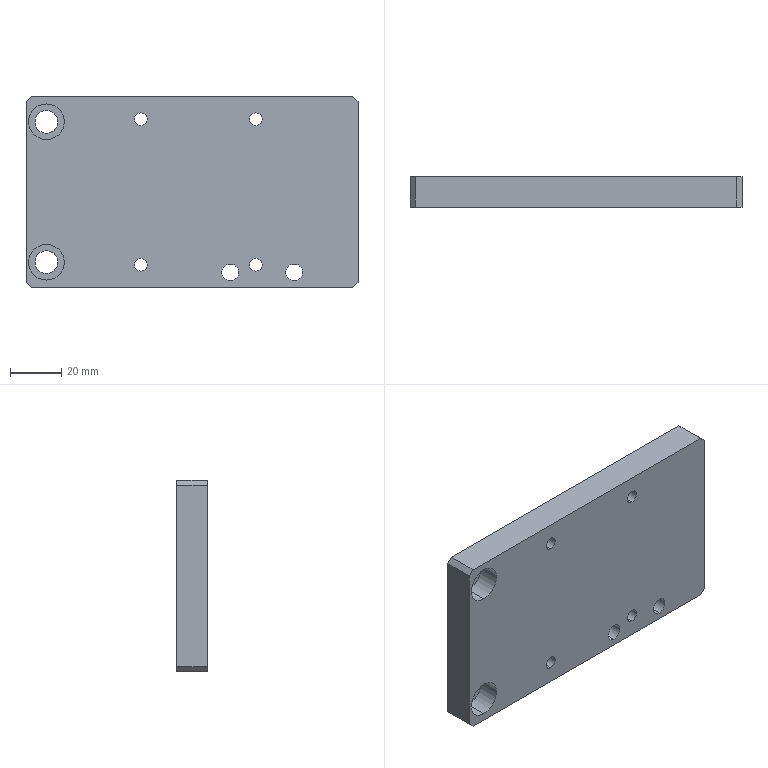Part | SolidWorks | features BaseBody 1 | 1 solid | 50 faces | box 130 x 12 x 75 mm | volume 110369 mm3 | cylinder 30 | plane 14 | cone 6 | commonest cylinder face diameters 5 x14 6.6 x4 9 x4 11 x4 14 x4
STEP:
#1=CARTESIAN_POINT('',(25.,0.,26.));
#2=VERTEX_POINT('',#1);
#3=CARTESIAN_POINT('',(25.,0.,31.));
#4=VERTEX_POINT('',#3);
#5=CARTESIAN_POINT('',(25.,0.,28.5));
#6=DIRECTION('',(0.,1.,0.));
#7=DIRECTION('',(0.,0.,1.));
#8=AXIS2_PLACEMENT_3D('',#5,#6,#7);
#9=CIRCLE('',#8,2.5);
#10=EDGE_CURVE('',#2,#4,#9,.T.);
#11=ORIENTED_EDGE('',*,*,#10,.F.);
#12=CARTESIAN_POINT('',(25.,12.,26.));
#13=VERTEX_POINT('',#12);
#14=CARTESIAN_POINT('',(25.,12.,26.));
#15=DIRECTION('',(0.,1.,0.));
#16=VECTOR('',#15,1000.);
#17=LINE('',#14,#16);
#18=EDGE_CURVE('',#2,#13,#17,.T.);
#19=ORIENTED_EDGE('',*,*,#18,.T.);
#20=CARTESIAN_POINT('',(25.,12.,31.));
#21=VERTEX_POINT('',#20);
#22=CARTESIAN_POINT('',(25.,12.,28.5));
#23=DIRECTION('',(0.,-1.,0.));
#24=DIRECTION('',(0.,0.,1.));
#25=AXIS2_PLACEMENT_3D('',#22,#23,#24);
#26=CIRCLE('',#25,2.5);
#27=EDGE_CURVE('',#21,#13,#26,.T.);
#28=ORIENTED_EDGE('',*,*,#27,.F.);
#29=CARTESIAN_POINT('',(25.,12.,31.));
#30=DIRECTION('',(0.,1.,0.));
#31=VECTOR('',#30,1000.);
#32=LINE('',#29,#31);
#33=EDGE_CURVE('',#4,#21,#32,.T.);
#34=ORIENTED_EDGE('',*,*,#33,.F.);
#35=EDGE_LOOP('',(#11,#19,#28,#34));
#36=FACE_OUTER_BOUND('',#35,.T.);
#37=CARTESIAN_POINT('',(25.,12.,28.5));
#38=DIRECTION('',(0.,1.,0.));
#39=DIRECTION('',(0.,0.,1.));
#40=AXIS2_PLACEMENT_3D('',#37,#38,#39);
#41=CYLINDRICAL_SURFACE('',#40,2.5);
#42=ADVANCED_FACE('',(#36),#41,.F.);
#43=CARTESIAN_POINT('',(-20.,0.,26.));
#44=VERTEX_POINT('',#43);
#45=CARTESIAN_POINT('',(-20.,0.,31.));
#46=VERTEX_POINT('',#45);
#47=CARTESIAN_POINT('',(-20.,0.,28.5));
#48=DIRECTION('',(0.,1.,0.));
#49=DIRECTION('',(0.,0.,1.));
#50=AXIS2_PLACEMENT_3D('',#47,#48,#49);
#51=CIRCLE('',#50,2.5);
#52=EDGE_CURVE('',#44,#46,#51,.T.);
#53=ORIENTED_EDGE('',*,*,#52,.F.);
#54=CARTESIAN_POINT('',(-20.,12.,26.));
#55=VERTEX_POINT('',#54);
#56=CARTESIAN_POINT('',(-20.,12.,26.));
#57=DIRECTION('',(0.,1.,0.));
#58=VECTOR('',#57,1000.);
#59=LINE('',#56,#58);
#60=EDGE_CURVE('',#44,#55,#59,.T.);
#61=ORIENTED_EDGE('',*,*,#60,.T.);
#62=CARTESIAN_POINT('',(-20.,12.,31.));
#63=VERTEX_POINT('',#62);
#64=CARTESIAN_POINT('',(-20.,12.,28.5));
#65=DIRECTION('',(0.,-1.,0.));
#66=DIRECTION('',(0.,0.,1.));
#67=AXIS2_PLACEMENT_3D('',#64,#65,#66);
#68=CIRCLE('',#67,2.5);
#69=EDGE_CURVE('',#63,#55,#68,.T.);
#70=ORIENTED_EDGE('',*,*,#69,.F.);
#71=CARTESIAN_POINT('',(-20.,12.,31.));
#72=DIRECTION('',(0.,1.,0.));
#73=VECTOR('',#72,1000.);
#74=LINE('',#71,#73);
#75=EDGE_CURVE('',#46,#63,#74,.T.);
#76=ORIENTED_EDGE('',*,*,#75,.F.);
#77=EDGE_LOOP('',(#53,#61,#70,#76));
#78=FACE_OUTER_BOUND('',#77,.T.);
#79=CARTESIAN_POINT('',(-20.,12.,28.5));
#80=DIRECTION('',(0.,1.,0.));
#81=DIRECTION('',(0.,0.,1.));
#82=AXIS2_PLACEMENT_3D('',#79,#80,#81);
#83=CYLINDRICAL_SURFACE('',#82,2.5);
#84=ADVANCED_FACE('',(#78),#83,.F.);
#85=CARTESIAN_POINT('',(25.,0.,-31.));
#86=VERTEX_POINT('',#85);
#87=CARTESIAN_POINT('',(25.,0.,-26.));
#88=VERTEX_POINT('',#87);
#89=CARTESIAN_POINT('',(25.,0.,-28.5));
#90=DIRECTION('',(0.,1.,0.));
#91=DIRECTION('',(0.,0.,1.));
#92=AXIS2_PLACEMENT_3D('',#89,#90,#91);
#93=CIRCLE('',#92,2.5);
#94=EDGE_CURVE('',#86,#88,#93,.T.);
#95=ORIENTED_EDGE('',*,*,#94,.F.);
#96=CARTESIAN_POINT('',(25.,12.,-31.));
#97=VERTEX_POINT('',#96);
#98=CARTESIAN_POINT('',(25.,12.,-31.));
#99=DIRECTION('',(0.,1.,0.));
#100=VECTOR('',#99,1000.);
#101=LINE('',#98,#100);
#102=EDGE_CURVE('',#86,#97,#101,.T.);
#103=ORIENTED_EDGE('',*,*,#102,.T.);
#104=CARTESIAN_POINT('',(25.,12.,-26.));
#105=VERTEX_POINT('',#104);
#106=CARTESIAN_POINT('',(25.,12.,-28.5));
#107=DIRECTION('',(0.,-1.,0.));
#108=DIRECTION('',(0.,0.,1.));
#109=AXIS2_PLACEMENT_3D('',#106,#107,#108);
#110=CIRCLE('',#109,2.5);
#111=EDGE_CURVE('',#105,#97,#110,.T.);
#112=ORIENTED_EDGE('',*,*,#111,.F.);
#113=CARTESIAN_POINT('',(25.,12.,-26.));
#114=DIRECTION('',(0.,1.,0.));
#115=VECTOR('',#114,1000.);
#116=LINE('',#113,#115);
#117=EDGE_CURVE('',#88,#105,#116,.T.);
#118=ORIENTED_EDGE('',*,*,#117,.F.);
#119=EDGE_LOOP('',(#95,#103,#112,#118));
#120=FACE_OUTER_BOUND('',#119,.T.);
#121=CARTESIAN_POINT('',(25.,12.,-28.5));
#122=DIRECTION('',(0.,1.,0.));
#123=DIRECTION('',(0.,0.,1.));
#124=AXIS2_PLACEMENT_3D('',#121,#122,#123);
#125=CYLINDRICAL_SURFACE('',#124,2.5);
#126=ADVANCED_FACE('',(#120),#125,.F.);
#127=CARTESIAN_POINT('',(-20.,0.,-31.));
#128=VERTEX_POINT('',#127);
#129=CARTESIAN_POINT('',(-20.,0.,-26.));
#130=VERTEX_POINT('',#129);
#131=CARTESIAN_POINT('',(-20.,0.,-28.5));
#132=DIRECTION('',(0.,1.,0.));
#133=DIRECTION('',(0.,0.,1.));
#134=AXIS2_PLACEMENT_3D('',#131,#132,#133);
#135=CIRCLE('',#134,2.5);
#136=EDGE_CURVE('',#128,#130,#135,.T.);
#137=ORIENTED_EDGE('',*,*,#136,.F.);
#138=CARTESIAN_POINT('',(-20.,12.,-31.));
#139=VERTEX_POINT('',#138);
#140=CARTESIAN_POINT('',(-20.,12.,-31.));
#141=DIRECTION('',(0.,1.,0.));
#142=VECTOR('',#141,1000.);
#143=LINE('',#140,#142);
#144=EDGE_CURVE('',#128,#139,#143,.T.);
#145=ORIENTED_EDGE('',*,*,#144,.T.);
#146=CARTESIAN_POINT('',(-20.,12.,-26.));
#147=VERTEX_POINT('',#146);
#148=CARTESIAN_POINT('',(-20.,12.,-28.5));
#149=DIRECTION('',(0.,-1.,0.));
#150=DIRECTION('',(0.,0.,1.));
#151=AXIS2_PLACEMENT_3D('',#148,#149,#150);
#152=CIRCLE('',#151,2.5);
#153=EDGE_CURVE('',#147,#139,#152,.T.);
#154=ORIENTED_EDGE('',*,*,#153,.F.);
#155=CARTESIAN_POINT('',(-20.,12.,-26.));
#156=DIRECTION('',(0.,1.,0.));
#157=VECTOR('',#156,1000.);
#158=LINE('',#155,#157);
#159=EDGE_CURVE('',#130,#147,#158,.T.);
#160=ORIENTED_EDGE('',*,*,#159,.F.);
#161=EDGE_LOOP('',(#137,#145,#154,#160));
#162=FACE_OUTER_BOUND('',#161,.T.);
#163=CARTESIAN_POINT('',(-20.,12.,-28.5));
#164=DIRECTION('',(0.,1.,0.));
#165=DIRECTION('',(0.,0.,1.));
#166=AXIS2_PLACEMENT_3D('',#163,#164,#165);
#167=CYLINDRICAL_SURFACE('',#166,2.5);
#168=ADVANCED_FACE('',(#162),#167,.F.);
#169=CARTESIAN_POINT('',(-57.,12.,32.));
#170=VERTEX_POINT('',#169);
#171=CARTESIAN_POINT('',(-57.,12.,23.));
#172=VERTEX_POINT('',#171);
#173=CARTESIAN_POINT('',(-57.,12.,27.5));
#174=DIRECTION('',(0.,-1.,0.));
#175=DIRECTION('',(0.,0.,-1.));
#176=AXIS2_PLACEMENT_3D('',#173,#174,#175);
#177=CIRCLE('',#176,4.5);
#178=EDGE_CURVE('',#170,#172,#177,.T.);
#179=ORIENTED_EDGE('',*,*,#178,.F.);
#180=CARTESIAN_POINT('',(-57.,8.6,32.));
#181=VERTEX_POINT('',#180);
#182=CARTESIAN_POINT('',(-57.,0.,32.));
#183=DIRECTION('',(0.,-1.,0.));
#184=VECTOR('',#183,1000.);
#185=LINE('',#182,#184);
#186=EDGE_CURVE('',#170,#181,#185,.T.);
#187=ORIENTED_EDGE('',*,*,#186,.T.);
#188=CARTESIAN_POINT('',(-57.,8.6,23.));
#189=VERTEX_POINT('',#188);
#190=CARTESIAN_POINT('',(-57.,8.6,27.5));
#191=DIRECTION('',(0.,1.,0.));
#192=DIRECTION('',(0.,0.,-1.));
#193=AXIS2_PLACEMENT_3D('',#190,#191,#192);
#194=CIRCLE('',#193,4.5);
#195=EDGE_CURVE('',#189,#181,#194,.T.);
#196=ORIENTED_EDGE('',*,*,#195,.F.);
#197=CARTESIAN_POINT('',(-57.,0.,23.));
#198=DIRECTION('',(0.,-1.,0.));
#199=VECTOR('',#198,1000.);
#200=LINE('',#197,#199);
#201=EDGE_CURVE('',#172,#189,#200,.T.);
#202=ORIENTED_EDGE('',*,*,#201,.F.);
#203=EDGE_LOOP('',(#179,#187,#196,#202));
#204=FACE_OUTER_BOUND('',#203,.T.);
#205=CARTESIAN_POINT('',(-57.,0.,27.5));
#206=DIRECTION('',(0.,-1.,0.));
#207=DIRECTION('',(0.,0.,-1.));
#208=AXIS2_PLACEMENT_3D('',#205,#206,#207);
#209=CYLINDRICAL_SURFACE('',#208,4.5);
#210=ADVANCED_FACE('',(#204),#209,.F.);
#211=CARTESIAN_POINT('',(-57.,12.,-23.));
#212=VERTEX_POINT('',#211);
#213=CARTESIAN_POINT('',(-57.,12.,-32.));
#214=VERTEX_POINT('',#213);
#215=CARTESIAN_POINT('',(-57.,12.,-27.5));
#216=DIRECTION('',(0.,-1.,0.));
#217=DIRECTION('',(0.,0.,-1.));
#218=AXIS2_PLACEMENT_3D('',#215,#216,#217);
#219=CIRCLE('',#218,4.5);
#220=EDGE_CURVE('',#212,#214,#219,.T.);
#221=ORIENTED_EDGE('',*,*,#220,.F.);
#222=CARTESIAN_POINT('',(-57.,8.6,-23.));
#223=VERTEX_POINT('',#222);
#224=CARTESIAN_POINT('',(-57.,0.,-23.));
#225=DIRECTION('',(0.,-1.,0.));
#226=VECTOR('',#225,1000.);
#227=LINE('',#224,#226);
#228=EDGE_CURVE('',#212,#223,#227,.T.);
#229=ORIENTED_EDGE('',*,*,#228,.T.);
#230=CARTESIAN_POINT('',(-57.,8.6,-32.));
#231=VERTEX_POINT('',#230);
#232=CARTESIAN_POINT('',(-57.,8.6,-27.5));
#233=DIRECTION('',(0.,1.,0.));
#234=DIRECTION('',(0.,0.,-1.));
#235=AXIS2_PLACEMENT_3D('',#232,#233,#234);
#236=CIRCLE('',#235,4.5);
#237=EDGE_CURVE('',#231,#223,#236,.T.);
#238=ORIENTED_EDGE('',*,*,#237,.F.);
#239=CARTESIAN_POINT('',(-57.,0.,-32.));
#240=DIRECTION('',(0.,-1.,0.));
#241=VECTOR('',#240,1000.);
#242=LINE('',#239,#241);
#243=EDGE_CURVE('',#214,#231,#242,.T.);
#244=ORIENTED_EDGE('',*,*,#243,.F.);
#245=EDGE_LOOP('',(#221,#229,#238,#244));
#246=FACE_OUTER_BOUND('',#245,.T.);
#247=CARTESIAN_POINT('',(-57.,0.,-27.5));
#248=DIRECTION('',(0.,-1.,0.));
#249=DIRECTION('',(0.,0.,-1.));
#250=AXIS2_PLACEMENT_3D('',#247,#248,#249);
#251=CYLINDRICAL_SURFACE('',#250,4.5);
#252=ADVANCED_FACE('',(#246),#251,.F.);
#253=CARTESIAN_POINT('',(40.,5.6,-37.));
#254=VERTEX_POINT('',#253);
#255=CARTESIAN_POINT('',(40.,5.6,-26.));
#256=VERTEX_POINT('',#255);
#257=CARTESIAN_POINT('',(40.,5.6,-31.5));
#258=DIRECTION('',(0.,1.,0.));
#259=DIRECTION('',(0.,0.,1.));
#260=AXIS2_PLACEMENT_3D('',#257,#258,#259);
#261=CIRCLE('',#260,5.5);
#262=EDGE_CURVE('',#254,#256,#261,.T.);
#263=ORIENTED_EDGE('',*,*,#262,.F.);
#264=CARTESIAN_POINT('',(40.,12.,-37.));
#265=VERTEX_POINT('',#264);
#266=CARTESIAN_POINT('',(40.,12.,-37.));
#267=DIRECTION('',(0.,1.,0.));
#268=VECTOR('',#267,1000.);
#269=LINE('',#266,#268);
#270=EDGE_CURVE('',#254,#265,#269,.T.);
#271=ORIENTED_EDGE('',*,*,#270,.T.);
#272=CARTESIAN_POINT('',(40.,12.,-26.));
#273=VERTEX_POINT('',#272);
#274=CARTESIAN_POINT('',(40.,12.,-31.5));
#275=DIRECTION('',(0.,-1.,0.));
#276=DIRECTION('',(0.,0.,1.));
#277=AXIS2_PLACEMENT_3D('',#274,#275,#276);
#278=CIRCLE('',#277,5.5);
#279=EDGE_CURVE('',#273,#265,#278,.T.);
#280=ORIENTED_EDGE('',*,*,#279,.F.);
#281=CARTESIAN_POINT('',(40.,12.,-26.));
#282=DIRECTION('',(0.,1.,0.));
#283=VECTOR('',#282,1000.);
#284=LINE('',#281,#283);
#285=EDGE_CURVE('',#256,#273,#284,.T.);
#286=ORIENTED_EDGE('',*,*,#285,.F.);
#287=EDGE_LOOP('',(#263,#271,#280,#286));
#288=FACE_OUTER_BOUND('',#287,.T.);
#289=CARTESIAN_POINT('',(40.,12.,-31.5));
#290=DIRECTION('',(0.,1.,0.));
#291=DIRECTION('',(0.,0.,1.));
#292=AXIS2_PLACEMENT_3D('',#289,#290,#291);
#293=CYLINDRICAL_SURFACE('',#292,5.5);
#294=ADVANCED_FACE('',(#288),#293,.F.);
#295=CARTESIAN_POINT('',(15.,5.6,-37.));
#296=VERTEX_POINT('',#295);
#297=CARTESIAN_POINT('',(15.,5.6,-26.));
#298=VERTEX_POINT('',#297);
#299=CARTESIAN_POINT('',(15.,5.6,-31.5));
#300=DIRECTION('',(0.,1.,0.));
#301=DIRECTION('',(0.,0.,1.));
#302=AXIS2_PLACEMENT_3D('',#299,#300,#301);
#303=CIRCLE('',#302,5.5);
#304=EDGE_CURVE('',#296,#298,#303,.T.);
#305=ORIENTED_EDGE('',*,*,#304,.F.);
#306=CARTESIAN_POINT('',(15.,12.,-37.));
#307=VERTEX_POINT('',#306);
#308=CARTESIAN_POINT('',(15.,12.,-37.));
#309=DIRECTION('',(0.,1.,0.));
#310=VECTOR('',#309,1000.);
#311=LINE('',#308,#310);
#312=EDGE_CURVE('',#296,#307,#311,.T.);
#313=ORIENTED_EDGE('',*,*,#312,.T.);
#314=CARTESIAN_POINT('',(15.,12.,-26.));
#315=VERTEX_POINT('',#314);
#316=CARTESIAN_POINT('',(15.,12.,-31.5));
#317=DIRECTION('',(0.,-1.,0.));
#318=DIRECTION('',(0.,0.,1.));
#319=AXIS2_PLACEMENT_3D('',#316,#317,#318);
#320=CIRCLE('',#319,5.5);
#321=EDGE_CURVE('',#315,#307,#320,.T.);
#322=ORIENTED_EDGE('',*,*,#321,.F.);
#323=CARTESIAN_POINT('',(15.,12.,-26.));
#324=DIRECTION('',(0.,1.,0.));
#325=VECTOR('',#324,1000.);
#326=LINE('',#323,#325);
#327=EDGE_CURVE('',#298,#315,#326,.T.);
#328=ORIENTED_EDGE('',*,*,#327,.F.);
#329=EDGE_LOOP('',(#305,#313,#322,#328));
#330=FACE_OUTER_BOUND('',#329,.T.);
#331=CARTESIAN_POINT('',(15.,12.,-31.5));
#332=DIRECTION('',(0.,1.,0.));
#333=DIRECTION('',(0.,0.,1.));
#334=AXIS2_PLACEMENT_3D('',#331,#332,#333);
#335=CYLINDRICAL_SURFACE('',#334,5.5);
#336=ADVANCED_FACE('',(#330),#335,.F.);
#337=CARTESIAN_POINT('',(50.,6.,-22.5));
#338=VERTEX_POINT('',#337);
#339=CARTESIAN_POINT('',(50.,6.,-27.5));
#340=VERTEX_POINT('',#339);
#341=CARTESIAN_POINT('',(50.,6.,-25.));
#342=DIRECTION('',(1.,0.,0.));
#343=DIRECTION('',(0.,0.,-1.));
#344=AXIS2_PLACEMENT_3D('',#341,#342,#343);
#345=CIRCLE('',#344,2.5);
#346=EDGE_CURVE('',#338,#340,#345,.T.);
#347=ORIENTED_EDGE('',*,*,#346,.F.);
#348=CARTESIAN_POINT('',(65.,6.,-22.5));
#349=VERTEX_POINT('',#348);
#350=CARTESIAN_POINT('',(65.,6.,-22.5));
#351=DIRECTION('',(1.,0.,0.));
#352=VECTOR('',#351,1000.);
#353=LINE('',#350,#352);
#354=EDGE_CURVE('',#338,#349,#353,.T.);
#355=ORIENTED_EDGE('',*,*,#354,.T.);
#356=CARTESIAN_POINT('',(65.,6.,-27.5));
#357=VERTEX_POINT('',#356);
#358=CARTESIAN_POINT('',(65.,6.,-25.));
#359=DIRECTION('',(1.,0.,0.));
#360=DIRECTION('',(0.,0.,-1.));
#361=AXIS2_PLACEMENT_3D('',#358,#359,#360);
#362=CIRCLE('',#361,2.5);
#363=EDGE_CURVE('',#349,#357,#362,.T.);
#364=ORIENTED_EDGE('',*,*,#363,.T.);
#365=CARTESIAN_POINT('',(65.,6.,-27.5));
#366=DIRECTION('',(1.,0.,0.));
#367=VECTOR('',#366,1000.);
#368=LINE('',#365,#367);
#369=EDGE_CURVE('',#340,#357,#368,.T.);
#370=ORIENTED_EDGE('',*,*,#369,.F.);
#371=EDGE_LOOP('',(#347,#355,#364,#370));
#372=FACE_OUTER_BOUND('',#371,.T.);
#373=CARTESIAN_POINT('',(65.,6.,-25.));
#374=DIRECTION('',(1.,0.,0.));
#375=DIRECTION('',(0.,0.,-1.));
#376=AXIS2_PLACEMENT_3D('',#373,#374,#375);
#377=CYLINDRICAL_SURFACE('',#376,2.5);
#378=ADVANCED_FACE('',(#372),#377,.F.);
#379=CARTESIAN_POINT('',(50.,6.,2.5));
#380=VERTEX_POINT('',#379);
#381=CARTESIAN_POINT('',(50.,6.,-2.5));
#382=VERTEX_POINT('',#381);
#383=CARTESIAN_POINT('',(50.,6.,0.));
#384=DIRECTION('',(1.,0.,0.));
#385=DIRECTION('',(0.,0.,-1.));
#386=AXIS2_PLACEMENT_3D('',#383,#384,#385);
#387=CIRCLE('',#386,2.5);
#388=EDGE_CURVE('',#380,#382,#387,.T.);
#389=ORIENTED_EDGE('',*,*,#388,.F.);
#390=CARTESIAN_POINT('',(65.,6.,2.5));
#391=VERTEX_POINT('',#390);
#392=CARTESIAN_POINT('',(65.,6.,2.5));
#393=DIRECTION('',(1.,0.,0.));
#394=VECTOR('',#393,1000.);
#395=LINE('',#392,#394);
#396=EDGE_CURVE('',#380,#391,#395,.T.);
#397=ORIENTED_EDGE('',*,*,#396,.T.);
#398=CARTESIAN_POINT('',(65.,6.,-2.5));
#399=VERTEX_POINT('',#398);
#400=CARTESIAN_POINT('',(65.,6.,0.));
#401=DIRECTION('',(1.,0.,0.));
#402=DIRECTION('',(0.,0.,-1.));
#403=AXIS2_PLACEMENT_3D('',#400,#401,#402);
#404=CIRCLE('',#403,2.5);
#405=EDGE_CURVE('',#391,#399,#404,.T.);
#406=ORIENTED_EDGE('',*,*,#405,.T.);
#407=CARTESIAN_POINT('',(65.,6.,-2.5));
#408=DIRECTION('',(1.,0.,0.));
#409=VECTOR('',#408,1000.);
#410=LINE('',#407,#409);
#411=EDGE_CURVE('',#382,#399,#410,.T.);
#412=ORIENTED_EDGE('',*,*,#411,.F.);
#413=EDGE_LOOP('',(#389,#397,#406,#412));
#414=FACE_OUTER_BOUND('',#413,.T.);
#415=CARTESIAN_POINT('',(65.,6.,0.));
#416=DIRECTION('',(1.,0.,0.));
#417=DIRECTION('',(0.,0.,-1.));
#418=AXIS2_PLACEMENT_3D('',#415,#416,#417);
#419=CYLINDRICAL_SURFACE('',#418,2.5);
#420=ADVANCED_FACE('',(#414),#419,.F.);
#421=CARTESIAN_POINT('',(50.,6.,27.5));
#422=VERTEX_POINT('',#421);
#423=CARTESIAN_POINT('',(50.,6.,22.5));
#424=VERTEX_POINT('',#423);
#425=CARTESIAN_POINT('',(50.,6.,25.));
#426=DIRECTION('',(1.,0.,0.));
#427=DIRECTION('',(0.,0.,-1.));
#428=AXIS2_PLACEMENT_3D('',#425,#426,#427);
#429=CIRCLE('',#428,2.5);
#430=EDGE_CURVE('',#422,#424,#429,.T.);
#431=ORIENTED_EDGE('',*,*,#430,.F.);
#432=CARTESIAN_POINT('',(65.,6.,27.5));
#433=VERTEX_POINT('',#432);
#434=CARTESIAN_POINT('',(65.,6.,27.5));
#435=DIRECTION('',(1.,0.,0.));
#436=VECTOR('',#435,1000.);
#437=LINE('',#434,#436);
#438=EDGE_CURVE('',#422,#433,#437,.T.);
#439=ORIENTED_EDGE('',*,*,#438,.T.);
#440=CARTESIAN_POINT('',(65.,6.,22.5));
#441=VERTEX_POINT('',#440);
#442=CARTESIAN_POINT('',(65.,6.,25.));
#443=DIRECTION('',(1.,0.,0.));
#444=DIRECTION('',(0.,0.,-1.));
#445=AXIS2_PLACEMENT_3D('',#442,#443,#444);
#446=CIRCLE('',#445,2.5);
#447=EDGE_CURVE('',#433,#441,#446,.T.);
#448=ORIENTED_EDGE('',*,*,#447,.T.);
#449=CARTESIAN_POINT('',(65.,6.,22.5));
#450=DIRECTION('',(1.,0.,0.));
#451=VECTOR('',#450,1000.);
#452=LINE('',#449,#451);
#453=EDGE_CURVE('',#424,#441,#452,.T.);
#454=ORIENTED_EDGE('',*,*,#453,.F.);
#455=EDGE_LOOP('',(#431,#439,#448,#454));
#456=FACE_OUTER_BOUND('',#455,.T.);
#457=CARTESIAN_POINT('',(65.,6.,25.));
#458=DIRECTION('',(1.,0.,0.));
#459=DIRECTION('',(0.,0.,-1.));
#460=AXIS2_PLACEMENT_3D('',#457,#458,#459);
#461=CYLINDRICAL_SURFACE('',#460,2.5);
#462=ADVANCED_FACE('',(#456),#461,.F.);
#463=CARTESIAN_POINT('',(-57.,8.6,20.5));
#464=VERTEX_POINT('',#463);
#465=CARTESIAN_POINT('',(-57.,8.6,34.5));
#466=VERTEX_POINT('',#465);
#467=CARTESIAN_POINT('',(-57.,8.6,27.5));
#468=DIRECTION('',(0.,1.,0.));
#469=DIRECTION('',(0.,0.,-1.));
#470=AXIS2_PLACEMENT_3D('',#467,#468,#469);
#471=CIRCLE('',#470,7.);
#472=EDGE_CURVE('',#464,#466,#471,.T.);
#473=ORIENTED_EDGE('',*,*,#472,.T.);
#474=CARTESIAN_POINT('',(-57.,0.,34.5));
#475=VERTEX_POINT('',#474);
#476=CARTESIAN_POINT('',(-57.,0.,34.5));
#477=DIRECTION('',(0.,-1.,0.));
#478=VECTOR('',#477,1000.);
#479=LINE('',#476,#478);
#480=EDGE_CURVE('',#466,#475,#479,.T.);
#481=ORIENTED_EDGE('',*,*,#480,.T.);
#482=CARTESIAN_POINT('',(-57.,0.,20.5));
#483=VERTEX_POINT('',#482);
#484=CARTESIAN_POINT('',(-57.,0.,27.5));
#485=DIRECTION('',(0.,-1.,0.));
#486=DIRECTION('',(0.,0.,-1.));
#487=AXIS2_PLACEMENT_3D('',#484,#485,#486);
#488=CIRCLE('',#487,7.);
#489=EDGE_CURVE('',#475,#483,#488,.T.);
#490=ORIENTED_EDGE('',*,*,#489,.T.);
#491=CARTESIAN_POINT('',(-57.,0.,20.5));
#492=DIRECTION('',(0.,-1.,0.));
#493=VECTOR('',#492,1000.);
#494=LINE('',#491,#493);
#495=EDGE_CURVE('',#464,#483,#494,.T.);
#496=ORIENTED_EDGE('',*,*,#495,.F.);
#497=EDGE_LOOP('',(#473,#481,#490,#496));
#498=FACE_OUTER_BOUND('',#497,.T.);
#499=CARTESIAN_POINT('',(-57.,0.,27.5));
#500=DIRECTION('',(0.,-1.,0.));
#501=DIRECTION('',(0.,0.,-1.));
#502=AXIS2_PLACEMENT_3D('',#499,#500,#501);
#503=CYLINDRICAL_SURFACE('',#502,7.);
#504=ADVANCED_FACE('',(#498),#503,.F.);
#505=CARTESIAN_POINT('',(-57.,8.6,-34.5));
#506=VERTEX_POINT('',#505);
#507=CARTESIAN_POINT('',(-57.,8.6,-20.5));
#508=VERTEX_POINT('',#507);
#509=CARTESIAN_POINT('',(-57.,8.6,-27.5));
#510=DIRECTION('',(0.,1.,0.));
#511=DIRECTION('',(0.,0.,-1.));
#512=AXIS2_PLACEMENT_3D('',#509,#510,#511);
#513=CIRCLE('',#512,7.);
#514=EDGE_CURVE('',#506,#508,#513,.T.);
#515=ORIENTED_EDGE('',*,*,#514,.T.);
#516=CARTESIAN_POINT('',(-57.,0.,-20.5));
#517=VERTEX_POINT('',#516);
#518=CARTESIAN_POINT('',(-57.,0.,-20.5));
#519=DIRECTION('',(0.,-1.,0.));
#520=VECTOR('',#519,1000.);
#521=LINE('',#518,#520);
#522=EDGE_CURVE('',#508,#517,#521,.T.);
#523=ORIENTED_EDGE('',*,*,#522,.T.);
#524=CARTESIAN_POINT('',(-57.,0.,-34.5));
#525=VERTEX_POINT('',#524);
#526=CARTESIAN_POINT('',(-57.,0.,-27.5));
#527=DIRECTION('',(0.,-1.,0.));
#528=DIRECTION('',(0.,0.,-1.));
#529=AXIS2_PLACEMENT_3D('',#526,#527,#528);
#530=CIRCLE('',#529,7.);
#531=EDGE_CURVE('',#517,#525,#530,.T.);
#532=ORIENTED_EDGE('',*,*,#531,.T.);
#533=CARTESIAN_POINT('',(-57.,0.,-34.5));
#534=DIRECTION('',(0.,-1.,0.));
#535=VECTOR('',#534,1000.);
#536=LINE('',#533,#535);
#537=EDGE_CURVE('',#506,#525,#536,.T.);
#538=ORIENTED_EDGE('',*,*,#537,.F.);
#539=EDGE_LOOP('',(#515,#523,#532,#538));
#540=FACE_OUTER_BOUND('',#539,.T.);
#541=CARTESIAN_POINT('',(-57.,0.,-27.5));
#542=DIRECTION('',(0.,-1.,0.));
#543=DIRECTION('',(0.,0.,-1.));
#544=AXIS2_PLACEMENT_3D('',#541,#542,#543);
#545=CYLINDRICAL_SURFACE('',#544,7.);
#546=ADVANCED_FACE('',(#540),#545,.F.);
#547=CARTESIAN_POINT('',(40.,0.,-28.2));
#548=VERTEX_POINT('',#547);
#549=CARTESIAN_POINT('',(40.,0.,-34.8));
#550=VERTEX_POINT('',#549);
#551=CARTESIAN_POINT('',(40.,0.,-31.5));
#552=DIRECTION('',(0.,-1.,0.));
#553=DIRECTION('',(0.,0.,1.));
#554=AXIS2_PLACEMENT_3D('',#551,#552,#553);
#555=CIRCLE('',#554,3.3);
#556=EDGE_CURVE('',#548,#550,#555,.T.);
#557=ORIENTED_EDGE('',*,*,#556,.T.);
#558=CARTESIAN_POINT('',(40.,5.6,-34.8));
#559=VERTEX_POINT('',#558);
#560=CARTESIAN_POINT('',(40.,12.,-34.8));
#561=DIRECTION('',(0.,1.,0.));
#562=VECTOR('',#561,1000.);
#563=LINE('',#560,#562);
#564=EDGE_CURVE('',#550,#559,#563,.T.);
#565=ORIENTED_EDGE('',*,*,#564,.T.);
#566=CARTESIAN_POINT('',(40.,5.6,-28.2));
#567=VERTEX_POINT('',#566);
#568=CARTESIAN_POINT('',(40.,5.6,-31.5));
#569=DIRECTION('',(0.,1.,0.));
#570=DIRECTION('',(0.,0.,1.));
#571=AXIS2_PLACEMENT_3D('',#568,#569,#570);
#572=CIRCLE('',#571,3.3);
#573=EDGE_CURVE('',#559,#567,#572,.T.);
#574=ORIENTED_EDGE('',*,*,#573,.T.);
#575=CARTESIAN_POINT('',(40.,12.,-28.2));
#576=DIRECTION('',(0.,1.,0.));
#577=VECTOR('',#576,1000.);
#578=LINE('',#575,#577);
#579=EDGE_CURVE('',#548,#567,#578,.T.);
#580=ORIENTED_EDGE('',*,*,#579,.F.);
#581=EDGE_LOOP('',(#557,#565,#574,#580));
#582=FACE_OUTER_BOUND('',#581,.T.);
#583=CARTESIAN_POINT('',(40.,12.,-31.5));
#584=DIRECTION('',(0.,1.,0.));
#585=DIRECTION('',(0.,0.,1.));
#586=AXIS2_PLACEMENT_3D('',#583,#584,#585);
#587=CYLINDRICAL_SURFACE('',#586,3.3);
#588=ADVANCED_FACE('',(#582),#587,.F.);
#589=CARTESIAN_POINT('',(15.,0.,-28.2));
#590=VERTEX_POINT('',#589);
#591=CARTESIAN_POINT('',(15.,0.,-34.8));
#592=VERTEX_POINT('',#591);
#593=CARTESIAN_POINT('',(15.,0.,-31.5));
#594=DIRECTION('',(0.,-1.,0.));
#595=DIRECTION('',(0.,0.,1.));
#596=AXIS2_PLACEMENT_3D('',#593,#594,#595);
#597=CIRCLE('',#596,3.3);
#598=EDGE_CURVE('',#590,#592,#597,.T.);
#599=ORIENTED_EDGE('',*,*,#598,.T.);
#600=CARTESIAN_POINT('',(15.,5.6,-34.8));
#601=VERTEX_POINT('',#600);
#602=CARTESIAN_POINT('',(15.,12.,-34.8));
#603=DIRECTION('',(0.,1.,0.));
#604=VECTOR('',#603,1000.);
#605=LINE('',#602,#604);
#606=EDGE_CURVE('',#592,#601,#605,.T.);
#607=ORIENTED_EDGE('',*,*,#606,.T.);
#608=CARTESIAN_POINT('',(15.,5.6,-28.2));
#609=VERTEX_POINT('',#608);
#610=CARTESIAN_POINT('',(15.,5.6,-31.5));
#611=DIRECTION('',(0.,1.,0.));
#612=DIRECTION('',(0.,0.,1.));
#613=AXIS2_PLACEMENT_3D('',#610,#611,#612);
#614=CIRCLE('',#613,3.3);
#615=EDGE_CURVE('',#601,#609,#614,.T.);
#616=ORIENTED_EDGE('',*,*,#615,.T.);
#617=CARTESIAN_POINT('',(15.,12.,-28.2));
#618=DIRECTION('',(0.,1.,0.));
#619=VECTOR('',#618,1000.);
#620=LINE('',#617,#619);
#621=EDGE_CURVE('',#590,#609,#620,.T.);
#622=ORIENTED_EDGE('',*,*,#621,.F.);
#623=EDGE_LOOP('',(#599,#607,#616,#622));
#624=FACE_OUTER_BOUND('',#623,.T.);
#625=CARTESIAN_POINT('',(15.,12.,-31.5));
#626=DIRECTION('',(0.,1.,0.));
#627=DIRECTION('',(0.,0.,1.));
#628=AXIS2_PLACEMENT_3D('',#625,#626,#627);
#629=CYLINDRICAL_SURFACE('',#628,3.3);
#630=ADVANCED_FACE('',(#624),#629,.F.);
#631=CARTESIAN_POINT('',(48.498,6.,-25.));
#632=VERTEX_POINT('',#631);
#633=CARTESIAN_POINT('',(50.,6.,-27.5));
#634=DIRECTION('',(0.515,0.,-0.8572));
#635=VECTOR('',#634,1000.);
#636=LINE('',#633,#635);
#637=EDGE_CURVE('',#632,#340,#636,.T.);
#638=ORIENTED_EDGE('',*,*,#637,.F.);
#639=CARTESIAN_POINT('',(50.,6.,-22.5));
#640=DIRECTION('',(0.515,0.,0.8572));
#641=VECTOR('',#640,1000.);
#642=LINE('',#639,#641);
#643=EDGE_CURVE('',#632,#338,#642,.T.);
#644=ORIENTED_EDGE('',*,*,#643,.T.);
#645=ORIENTED_EDGE('',*,*,#346,.T.);
#646=EDGE_LOOP('',(#638,#644,#645));
#647=FACE_OUTER_BOUND('',#646,.T.);
#648=CARTESIAN_POINT('',(50.,6.,-25.));
#649=DIRECTION('',(1.,0.,0.));
#650=DIRECTION('',(0.,0.,-1.));
#651=AXIS2_PLACEMENT_3D('',#648,#649,#650);
#652=CONICAL_SURFACE('',#651,2.5,1.03);
#653=ADVANCED_FACE('',(#647),#652,.F.);
#654=CARTESIAN_POINT('',(48.498,6.,0.));
#655=VERTEX_POINT('',#654);
#656=CARTESIAN_POINT('',(50.,6.,-2.5));
#657=DIRECTION('',(0.515,0.,-0.8572));
#658=VECTOR('',#657,1000.);
#659=LINE('',#656,#658);
#660=EDGE_CURVE('',#655,#382,#659,.T.);
#661=ORIENTED_EDGE('',*,*,#660,.F.);
#662=CARTESIAN_POINT('',(50.,6.,2.5));
#663=DIRECTION('',(0.515,0.,0.8572));
#664=VECTOR('',#663,1000.);
#665=LINE('',#662,#664);
#666=EDGE_CURVE('',#655,#380,#665,.T.);
#667=ORIENTED_EDGE('',*,*,#666,.T.);
#668=ORIENTED_EDGE('',*,*,#388,.T.);
#669=EDGE_LOOP('',(#661,#667,#668));
#670=FACE_OUTER_BOUND('',#669,.T.);
#671=CARTESIAN_POINT('',(50.,6.,0.));
#672=DIRECTION('',(1.,0.,0.));
#673=DIRECTION('',(0.,0.,-1.));
#674=AXIS2_PLACEMENT_3D('',#671,#672,#673);
#675=CONICAL_SURFACE('',#674,2.5,1.03);
#676=ADVANCED_FACE('',(#670),#675,.F.);
#677=CARTESIAN_POINT('',(48.498,6.,25.));
#678=VERTEX_POINT('',#677);
#679=CARTESIAN_POINT('',(50.,6.,22.5));
#680=DIRECTION('',(0.515,0.,-0.8572));
#681=VECTOR('',#680,1000.);
#682=LINE('',#679,#681);
#683=EDGE_CURVE('',#678,#424,#682,.T.);
#684=ORIENTED_EDGE('',*,*,#683,.F.);
#685=CARTESIAN_POINT('',(50.,6.,27.5));
#686=DIRECTION('',(0.515,0.,0.8572));
#687=VECTOR('',#686,1000.);
#688=LINE('',#685,#687);
#689=EDGE_CURVE('',#678,#422,#688,.T.);
#690=ORIENTED_EDGE('',*,*,#689,.T.);
#691=ORIENTED_EDGE('',*,*,#430,.T.);
#692=EDGE_LOOP('',(#684,#690,#691));
#693=FACE_OUTER_BOUND('',#692,.T.);
#694=CARTESIAN_POINT('',(50.,6.,25.));
#695=DIRECTION('',(1.,0.,0.));
#696=DIRECTION('',(0.,0.,-1.));
#697=AXIS2_PLACEMENT_3D('',#694,#695,#696);
#698=CONICAL_SURFACE('',#697,2.5,1.03);
#699=ADVANCED_FACE('',(#693),#698,.F.);
#700=CARTESIAN_POINT('',(-63.,12.,37.5));
#701=VERTEX_POINT('',#700);
#702=CARTESIAN_POINT('',(63.,12.,37.5));
#703=VERTEX_POINT('',#702);
#704=CARTESIAN_POINT('',(0.,12.,37.5));
#705=DIRECTION('',(1.,0.,0.));
#706=VECTOR('',#705,1000.);
#707=LINE('',#704,#706);
#708=EDGE_CURVE('',#701,#703,#707,.T.);
#709=ORIENTED_EDGE('',*,*,#708,.T.);
#710=CARTESIAN_POINT('',(65.,12.,35.5));
#711=VERTEX_POINT('',#710);
#712=CARTESIAN_POINT('',(63.,12.,37.5));
#713=DIRECTION('',(0.7071,0.,-0.7071));
#714=VECTOR('',#713,1000.);
#715=LINE('',#712,#714);
#716=EDGE_CURVE('',#703,#711,#715,.T.);
#717=ORIENTED_EDGE('',*,*,#716,.T.);
#718=CARTESIAN_POINT('',(65.,12.,-35.5));
#719=VERTEX_POINT('',#718);
#720=CARTESIAN_POINT('',(65.,12.,0.));
#721=DIRECTION('',(0.,0.,-1.));
#722=VECTOR('',#721,1000.);
#723=LINE('',#720,#722);
#724=EDGE_CURVE('',#711,#719,#723,.T.);
#725=ORIENTED_EDGE('',*,*,#724,.T.);
#726=CARTESIAN_POINT('',(63.,12.,-37.5));
#727=VERTEX_POINT('',#726);
#728=CARTESIAN_POINT('',(65.,12.,-35.5));
#729=DIRECTION('',(-0.7071,0.,-0.7071));
#730=VECTOR('',#729,1000.);
#731=LINE('',#728,#730);
#732=EDGE_CURVE('',#719,#727,#731,.T.);
#733=ORIENTED_EDGE('',*,*,#732,.T.);
#734=CARTESIAN_POINT('',(-63.,12.,-37.5));
#735=VERTEX_POINT('',#734);
#736=CARTESIAN_POINT('',(0.,12.,-37.5));
#737=DIRECTION('',(-1.,0.,0.));
#738=VECTOR('',#737,1000.);
#739=LINE('',#736,#738);
#740=EDGE_CURVE('',#727,#735,#739,.T.);
#741=ORIENTED_EDGE('',*,*,#740,.T.);
#742=CARTESIAN_POINT('',(-65.,12.,-35.5));
#743=VERTEX_POINT('',#742);
#744=CARTESIAN_POINT('',(-63.,12.,-37.5));
#745=DIRECTION('',(-0.7071,0.,0.7071));
#746=VECTOR('',#745,1000.);
#747=LINE('',#744,#746);
#748=EDGE_CURVE('',#735,#743,#747,.T.);
#749=ORIENTED_EDGE('',*,*,#748,.T.);
#750=CARTESIAN_POINT('',(-65.,12.,35.5));
#751=VERTEX_POINT('',#750);
#752=CARTESIAN_POINT('',(-65.,12.,0.));
#753=DIRECTION('',(0.,0.,1.));
#754=VECTOR('',#753,1000.);
#755=LINE('',#752,#754);
#756=EDGE_CURVE('',#743,#751,#755,.T.);
#757=ORIENTED_EDGE('',*,*,#756,.T.);
#758=CARTESIAN_POINT('',(-65.,12.,35.5));
#759=DIRECTION('',(0.7071,0.,0.7071));
#760=VECTOR('',#759,1000.);
#761=LINE('',#758,#760);
#762=EDGE_CURVE('',#751,#701,#761,.T.);
#763=ORIENTED_EDGE('',*,*,#762,.T.);
#764=EDGE_LOOP('',(#709,#717,#725,#733,#741,#749,#757,#763));
#765=FACE_OUTER_BOUND('',#764,.T.);
#766=ORIENTED_EDGE('',*,*,#27,.T.);
#767=CARTESIAN_POINT('',(25.,12.,28.5));
#768=DIRECTION('',(0.,-1.,0.));
#769=DIRECTION('',(0.,0.,1.));
#770=AXIS2_PLACEMENT_3D('',#767,#768,#769);
#771=CIRCLE('',#770,2.5);
#772=EDGE_CURVE('',#13,#21,#771,.T.);
#773=ORIENTED_EDGE('',*,*,#772,.T.);
#774=EDGE_LOOP('',(#766,#773));
#775=FACE_BOUND('',#774,.T.);
#776=ORIENTED_EDGE('',*,*,#69,.T.);
#777=CARTESIAN_POINT('',(-20.,12.,28.5));
#778=DIRECTION('',(0.,-1.,0.));
#779=DIRECTION('',(0.,0.,1.));
#780=AXIS2_PLACEMENT_3D('',#777,#778,#779);
#781=CIRCLE('',#780,2.5);
#782=EDGE_CURVE('',#55,#63,#781,.T.);
#783=ORIENTED_EDGE('',*,*,#782,.T.);
#784=EDGE_LOOP('',(#776,#783));
#785=FACE_BOUND('',#784,.T.);
#786=ORIENTED_EDGE('',*,*,#111,.T.);
#787=CARTESIAN_POINT('',(25.,12.,-28.5));
#788=DIRECTION('',(0.,-1.,0.));
#789=DIRECTION('',(0.,0.,1.));
#790=AXIS2_PLACEMENT_3D('',#787,#788,#789);
#791=CIRCLE('',#790,2.5);
#792=EDGE_CURVE('',#97,#105,#791,.T.);
#793=ORIENTED_EDGE('',*,*,#792,.T.);
#794=EDGE_LOOP('',(#786,#793));
#795=FACE_BOUND('',#794,.T.);
#796=ORIENTED_EDGE('',*,*,#153,.T.);
#797=CARTESIAN_POINT('',(-20.,12.,-28.5));
#798=DIRECTION('',(0.,-1.,0.));
#799=DIRECTION('',(0.,0.,1.));
#800=AXIS2_PLACEMENT_3D('',#797,#798,#799);
#801=CIRCLE('',#800,2.5);
#802=EDGE_CURVE('',#139,#147,#801,.T.);
#803=ORIENTED_EDGE('',*,*,#802,.T.);
#804=EDGE_LOOP('',(#796,#803));
#805=FACE_BOUND('',#804,.T.);
#806=CARTESIAN_POINT('',(-57.,12.,27.5));
#807=DIRECTION('',(0.,-1.,0.));
#808=DIRECTION('',(0.,0.,-1.));
#809=AXIS2_PLACEMENT_3D('',#806,#807,#808);
#810=CIRCLE('',#809,4.5);
#811=EDGE_CURVE('',#172,#170,#810,.T.);
#812=ORIENTED_EDGE('',*,*,#811,.T.);
#813=ORIENTED_EDGE('',*,*,#178,.T.);
#814=EDGE_LOOP('',(#812,#813));
#815=FACE_BOUND('',#814,.T.);
#816=CARTESIAN_POINT('',(-57.,12.,-27.5));
#817=DIRECTION('',(0.,-1.,0.));
#818=DIRECTION('',(0.,0.,-1.));
#819=AXIS2_PLACEMENT_3D('',#816,#817,#818);
#820=CIRCLE('',#819,4.5);
#821=EDGE_CURVE('',#214,#212,#820,.T.);
#822=ORIENTED_EDGE('',*,*,#821,.T.);
#823=ORIENTED_EDGE('',*,*,#220,.T.);
#824=EDGE_LOOP('',(#822,#823));
#825=FACE_BOUND('',#824,.T.);
#826=ORIENTED_EDGE('',*,*,#279,.T.);
#827=CARTESIAN_POINT('',(40.,12.,-31.5));
#828=DIRECTION('',(0.,-1.,0.));
#829=DIRECTION('',(0.,0.,1.));
#830=AXIS2_PLACEMENT_3D('',#827,#828,#829);
#831=CIRCLE('',#830,5.5);
#832=EDGE_CURVE('',#265,#273,#831,.T.);
#833=ORIENTED_EDGE('',*,*,#832,.T.);
#834=EDGE_LOOP('',(#826,#833));
#835=FACE_BOUND('',#834,.T.);
#836=ORIENTED_EDGE('',*,*,#321,.T.);
#837=CARTESIAN_POINT('',(15.,12.,-31.5));
#838=DIRECTION('',(0.,-1.,0.));
#839=DIRECTION('',(0.,0.,1.));
#840=AXIS2_PLACEMENT_3D('',#837,#838,#839);
#841=CIRCLE('',#840,5.5);
#842=EDGE_CURVE('',#307,#315,#841,.T.);
#843=ORIENTED_EDGE('',*,*,#842,.T.);
#844=EDGE_LOOP('',(#836,#843));
#845=FACE_BOUND('',#844,.T.);
#846=CARTESIAN_POINT('',(0.,12.,0.));
#847=DIRECTION('',(0.,1.,0.));
#848=DIRECTION('',(0.,0.,1.));
#849=AXIS2_PLACEMENT_3D('',#846,#847,#848);
#850=PLANE('',#849);
#851=ADVANCED_FACE('',(#765,#775,#785,#795,#805,#815,#825,#835,#845),#850,.T.);
#852=CARTESIAN_POINT('',(63.,0.,37.5));
#853=VERTEX_POINT('',#852);
#854=CARTESIAN_POINT('',(63.,12.,37.5));
#855=DIRECTION('',(0.,1.,0.));
#856=VECTOR('',#855,1000.);
#857=LINE('',#854,#856);
#858=EDGE_CURVE('',#853,#703,#857,.T.);
#859=ORIENTED_EDGE('',*,*,#858,.F.);
#860=CARTESIAN_POINT('',(65.,0.,35.5));
#861=VERTEX_POINT('',#860);
#862=CARTESIAN_POINT('',(65.,0.,35.5));
#863=DIRECTION('',(-0.7071,0.,0.7071));
#864=VECTOR('',#863,1000.);
#865=LINE('',#862,#864);
#866=EDGE_CURVE('',#861,#853,#865,.T.);
#867=ORIENTED_EDGE('',*,*,#866,.F.);
#868=CARTESIAN_POINT('',(65.,12.,35.5));
#869=DIRECTION('',(0.,-1.,0.));
#870=VECTOR('',#869,1000.);
#871=LINE('',#868,#870);
#872=EDGE_CURVE('',#711,#861,#871,.T.);
#873=ORIENTED_EDGE('',*,*,#872,.F.);
#874=ORIENTED_EDGE('',*,*,#716,.F.);
#875=EDGE_LOOP('',(#859,#867,#873,#874));
#876=FACE_OUTER_BOUND('',#875,.T.);
#877=CARTESIAN_POINT('',(65.,12.,35.5));
#878=DIRECTION('',(-0.7071,0.,-0.7071));
#879=DIRECTION('',(-0.7071,0.,0.7071));
#880=AXIS2_PLACEMENT_3D('',#877,#878,#879);
#881=PLANE('',#880);
#882=ADVANCED_FACE('',(#876),#881,.F.);
#883=ORIENTED_EDGE('',*,*,#858,.T.);
#884=ORIENTED_EDGE('',*,*,#708,.F.);
#885=CARTESIAN_POINT('',(-63.,0.,37.5));
#886=VERTEX_POINT('',#885);
#887=CARTESIAN_POINT('',(-63.,12.,37.5));
#888=DIRECTION('',(0.,1.,0.));
#889=VECTOR('',#888,1000.);
#890=LINE('',#887,#889);
#891=EDGE_CURVE('',#886,#701,#890,.T.);
#892=ORIENTED_EDGE('',*,*,#891,.F.);
#893=CARTESIAN_POINT('',(-65.,0.,37.5));
#894=DIRECTION('',(-1.,0.,0.));
#895=VECTOR('',#894,1000.);
#896=LINE('',#893,#895);
#897=EDGE_CURVE('',#853,#886,#896,.T.);
#898=ORIENTED_EDGE('',*,*,#897,.F.);
#899=EDGE_LOOP('',(#883,#884,#892,#898));
#900=FACE_OUTER_BOUND('',#899,.T.);
#901=CARTESIAN_POINT('',(-65.,12.,37.5));
#902=DIRECTION('',(0.,0.,-1.));
#903=DIRECTION('',(-1.,0.,0.));
#904=AXIS2_PLACEMENT_3D('',#901,#902,#903);
#905=PLANE('',#904);
#906=ADVANCED_FACE('',(#900),#905,.F.);
#907=CARTESIAN_POINT('',(-65.,0.,35.5));
#908=VERTEX_POINT('',#907);
#909=CARTESIAN_POINT('',(-65.,12.,35.5));
#910=DIRECTION('',(0.,1.,0.));
#911=VECTOR('',#910,1000.);
#912=LINE('',#909,#911);
#913=EDGE_CURVE('',#908,#751,#912,.T.);
#914=ORIENTED_EDGE('',*,*,#913,.F.);
#915=CARTESIAN_POINT('',(-63.,0.,37.5));
#916=DIRECTION('',(-0.7071,0.,-0.7071));
#917=VECTOR('',#916,1000.);
#918=LINE('',#915,#917);
#919=EDGE_CURVE('',#886,#908,#918,.T.);
#920=ORIENTED_EDGE('',*,*,#919,.F.);
#921=ORIENTED_EDGE('',*,*,#891,.T.);
#922=ORIENTED_EDGE('',*,*,#762,.F.);
#923=EDGE_LOOP('',(#914,#920,#921,#922));
#924=FACE_OUTER_BOUND('',#923,.T.);
#925=CARTESIAN_POINT('',(-63.,12.,37.5));
#926=DIRECTION('',(0.7071,0.,-0.7071));
#927=DIRECTION('',(-0.7071,0.,-0.7071));
#928=AXIS2_PLACEMENT_3D('',#925,#926,#927);
#929=PLANE('',#928);
#930=ADVANCED_FACE('',(#924),#929,.F.);
#931=CARTESIAN_POINT('',(-65.,0.,-35.5));
#932=VERTEX_POINT('',#931);
#933=CARTESIAN_POINT('',(-65.,12.,-35.5));
#934=DIRECTION('',(0.,1.,0.));
#935=VECTOR('',#934,1000.);
#936=LINE('',#933,#935);
#937=EDGE_CURVE('',#932,#743,#936,.T.);
#938=ORIENTED_EDGE('',*,*,#937,.F.);
#939=CARTESIAN_POINT('',(-65.,0.,-37.5));
#940=DIRECTION('',(0.,0.,-1.));
#941=VECTOR('',#940,1000.);
#942=LINE('',#939,#941);
#943=EDGE_CURVE('',#908,#932,#942,.T.);
#944=ORIENTED_EDGE('',*,*,#943,.F.);
#945=ORIENTED_EDGE('',*,*,#913,.T.);
#946=ORIENTED_EDGE('',*,*,#756,.F.);
#947=EDGE_LOOP('',(#938,#944,#945,#946));
#948=FACE_OUTER_BOUND('',#947,.T.);
#949=CARTESIAN_POINT('',(-65.,12.,-37.5));
#950=DIRECTION('',(1.,0.,0.));
#951=DIRECTION('',(0.,0.,-1.));
#952=AXIS2_PLACEMENT_3D('',#949,#950,#951);
#953=PLANE('',#952);
#954=ADVANCED_FACE('',(#948),#953,.F.);
#955=CARTESIAN_POINT('',(-63.,0.,-37.5));
#956=VERTEX_POINT('',#955);
#957=CARTESIAN_POINT('',(-63.,12.,-37.5));
#958=DIRECTION('',(0.,1.,0.));
#959=VECTOR('',#958,1000.);
#960=LINE('',#957,#959);
#961=EDGE_CURVE('',#956,#735,#960,.T.);
#962=ORIENTED_EDGE('',*,*,#961,.F.);
#963=CARTESIAN_POINT('',(-65.,0.,-35.5));
#964=DIRECTION('',(0.7071,0.,-0.7071));
#965=VECTOR('',#964,1000.);
#966=LINE('',#963,#965);
#967=EDGE_CURVE('',#932,#956,#966,.T.);
#968=ORIENTED_EDGE('',*,*,#967,.F.);
#969=ORIENTED_EDGE('',*,*,#937,.T.);
#970=ORIENTED_EDGE('',*,*,#748,.F.);
#971=EDGE_LOOP('',(#962,#968,#969,#970));
#972=FACE_OUTER_BOUND('',#971,.T.);
#973=CARTESIAN_POINT('',(-65.,12.,-35.5));
#974=DIRECTION('',(0.7071,0.,0.7071));
#975=DIRECTION('',(0.7071,0.,-0.7071));
#976=AXIS2_PLACEMENT_3D('',#973,#974,#975);
#977=PLANE('',#976);
#978=ADVANCED_FACE('',(#972),#977,.F.);
#979=CARTESIAN_POINT('',(63.,0.,-37.5));
#980=VERTEX_POINT('',#979);
#981=CARTESIAN_POINT('',(63.,12.,-37.5));
#982=DIRECTION('',(0.,1.,0.));
#983=VECTOR('',#982,1000.);
#984=LINE('',#981,#983);
#985=EDGE_CURVE('',#980,#727,#984,.T.);
#986=ORIENTED_EDGE('',*,*,#985,.F.);
#987=CARTESIAN_POINT('',(-65.,0.,-37.5));
#988=DIRECTION('',(1.,0.,0.));
#989=VECTOR('',#988,1000.);
#990=LINE('',#987,#989);
#991=EDGE_CURVE('',#956,#980,#990,.T.);
#992=ORIENTED_EDGE('',*,*,#991,.F.);
#993=ORIENTED_EDGE('',*,*,#961,.T.);
#994=ORIENTED_EDGE('',*,*,#740,.F.);
#995=EDGE_LOOP('',(#986,#992,#993,#994));
#996=FACE_OUTER_BOUND('',#995,.T.);
#997=CARTESIAN_POINT('',(-65.,12.,-37.5));
#998=DIRECTION('',(0.,0.,1.));
#999=DIRECTION('',(1.,0.,0.));
#1000=AXIS2_PLACEMENT_3D('',#997,#998,#999);
#1001=PLANE('',#1000);
#1002=ADVANCED_FACE('',(#996),#1001,.F.);
#1003=CARTESIAN_POINT('',(65.,0.,-35.5));
#1004=VERTEX_POINT('',#1003);
#1005=CARTESIAN_POINT('',(65.,12.,-35.5));
#1006=DIRECTION('',(0.,1.,0.));
#1007=VECTOR('',#1006,1000.);
#1008=LINE('',#1005,#1007);
#1009=EDGE_CURVE('',#1004,#719,#1008,.T.);
#1010=ORIENTED_EDGE('',*,*,#1009,.F.);
#1011=CARTESIAN_POINT('',(63.,0.,-37.5));
#1012=DIRECTION('',(0.7071,0.,0.7071));
#1013=VECTOR('',#1012,1000.);
#1014=LINE('',#1011,#1013);
#1015=EDGE_CURVE('',#980,#1004,#1014,.T.);
#1016=ORIENTED_EDGE('',*,*,#1015,.F.);
#1017=ORIENTED_EDGE('',*,*,#985,.T.);
#1018=ORIENTED_EDGE('',*,*,#732,.F.);
#1019=EDGE_LOOP('',(#1010,#1016,#1017,#1018));
#1020=FACE_OUTER_BOUND('',#1019,.T.);
#1021=CARTESIAN_POINT('',(63.,12.,-37.5));
#1022=DIRECTION('',(-0.7071,0.,0.7071));
#1023=DIRECTION('',(0.7071,0.,0.7071));
#1024=AXIS2_PLACEMENT_3D('',#1021,#1022,#1023);
#1025=PLANE('',#1024);
#1026=ADVANCED_FACE('',(#1020),#1025,.F.);
#1027=ORIENTED_EDGE('',*,*,#1009,.T.);
#1028=ORIENTED_EDGE('',*,*,#724,.F.);
#1029=ORIENTED_EDGE('',*,*,#872,.T.);
#1030=CARTESIAN_POINT('',(65.,0.,-37.5));
#1031=DIRECTION('',(0.,0.,1.));
#1032=VECTOR('',#1031,1000.);
#1033=LINE('',#1030,#1032);
#1034=EDGE_CURVE('',#1004,#861,#1033,.T.);
#1035=ORIENTED_EDGE('',*,*,#1034,.F.);
#1036=EDGE_LOOP('',(#1027,#1028,#1029,#1035));
#1037=FACE_OUTER_BOUND('',#1036,.T.);
#1038=CARTESIAN_POINT('',(65.,6.,-25.));
#1039=DIRECTION('',(1.,0.,0.));
#1040=DIRECTION('',(0.,0.,-1.));
#1041=AXIS2_PLACEMENT_3D('',#1038,#1039,#1040);
#1042=CIRCLE('',#1041,2.5);
#1043=EDGE_CURVE('',#357,#349,#1042,.T.);
#1044=ORIENTED_EDGE('',*,*,#1043,.F.);
#1045=ORIENTED_EDGE('',*,*,#363,.F.);
#1046=EDGE_LOOP('',(#1044,#1045));
#1047=FACE_BOUND('',#1046,.T.);
#1048=CARTESIAN_POINT('',(65.,6.,0.));
#1049=DIRECTION('',(1.,0.,0.));
#1050=DIRECTION('',(0.,0.,-1.));
#1051=AXIS2_PLACEMENT_3D('',#1048,#1049,#1050);
#1052=CIRCLE('',#1051,2.5);
#1053=EDGE_CURVE('',#399,#391,#1052,.T.);
#1054=ORIENTED_EDGE('',*,*,#1053,.F.);
#1055=ORIENTED_EDGE('',*,*,#405,.F.);
#1056=EDGE_LOOP('',(#1054,#1055));
#1057=FACE_BOUND('',#1056,.T.);
#1058=CARTESIAN_POINT('',(65.,6.,25.));
#1059=DIRECTION('',(1.,0.,0.));
#1060=DIRECTION('',(0.,0.,-1.));
#1061=AXIS2_PLACEMENT_3D('',#1058,#1059,#1060);
#1062=CIRCLE('',#1061,2.5);
#1063=EDGE_CURVE('',#441,#433,#1062,.T.);
#1064=ORIENTED_EDGE('',*,*,#1063,.F.);
#1065=ORIENTED_EDGE('',*,*,#447,.F.);
#1066=EDGE_LOOP('',(#1064,#1065));
#1067=FACE_BOUND('',#1066,.T.);
#1068=CARTESIAN_POINT('',(65.,12.,-37.5));
#1069=DIRECTION('',(-1.,0.,0.));
#1070=DIRECTION('',(0.,0.,1.));
#1071=AXIS2_PLACEMENT_3D('',#1068,#1069,#1070);
#1072=PLANE('',#1071);
#1073=ADVANCED_FACE('',(#1037,#1047,#1057,#1067),#1072,.F.);
#1074=ORIENTED_EDGE('',*,*,#18,.F.);
#1075=CARTESIAN_POINT('',(25.,0.,28.5));
#1076=DIRECTION('',(0.,1.,0.));
#1077=DIRECTION('',(0.,0.,1.));
#1078=AXIS2_PLACEMENT_3D('',#1075,#1076,#1077);
#1079=CIRCLE('',#1078,2.5);
#1080=EDGE_CURVE('',#4,#2,#1079,.T.);
#1081=ORIENTED_EDGE('',*,*,#1080,.F.);
#1082=ORIENTED_EDGE('',*,*,#33,.T.);
#1083=ORIENTED_EDGE('',*,*,#772,.F.);
#1084=EDGE_LOOP('',(#1074,#1081,#1082,#1083));
#1085=FACE_OUTER_BOUND('',#1084,.T.);
#1086=CARTESIAN_POINT('',(25.,12.,28.5));
#1087=DIRECTION('',(0.,1.,0.));
#1088=DIRECTION('',(0.,0.,1.));
#1089=AXIS2_PLACEMENT_3D('',#1086,#1087,#1088);
#1090=CYLINDRICAL_SURFACE('',#1089,2.5);
#1091=ADVANCED_FACE('',(#1085),#1090,.F.);
#1092=ORIENTED_EDGE('',*,*,#60,.F.);
#1093=CARTESIAN_POINT('',(-20.,0.,28.5));
#1094=DIRECTION('',(0.,1.,0.));
#1095=DIRECTION('',(0.,0.,1.));
#1096=AXIS2_PLACEMENT_3D('',#1093,#1094,#1095);
#1097=CIRCLE('',#1096,2.5);
#1098=EDGE_CURVE('',#46,#44,#1097,.T.);
#1099=ORIENTED_EDGE('',*,*,#1098,.F.);
#1100=ORIENTED_EDGE('',*,*,#75,.T.);
#1101=ORIENTED_EDGE('',*,*,#782,.F.);
#1102=EDGE_LOOP('',(#1092,#1099,#1100,#1101));
#1103=FACE_OUTER_BOUND('',#1102,.T.);
#1104=CARTESIAN_POINT('',(-20.,12.,28.5));
#1105=DIRECTION('',(0.,1.,0.));
#1106=DIRECTION('',(0.,0.,1.));
#1107=AXIS2_PLACEMENT_3D('',#1104,#1105,#1106);
#1108=CYLINDRICAL_SURFACE('',#1107,2.5);
#1109=ADVANCED_FACE('',(#1103),#1108,.F.);
#1110=ORIENTED_EDGE('',*,*,#102,.F.);
#1111=CARTESIAN_POINT('',(25.,0.,-28.5));
#1112=DIRECTION('',(0.,1.,0.));
#1113=DIRECTION('',(0.,0.,1.));
#1114=AXIS2_PLACEMENT_3D('',#1111,#1112,#1113);
#1115=CIRCLE('',#1114,2.5);
#1116=EDGE_CURVE('',#88,#86,#1115,.T.);
#1117=ORIENTED_EDGE('',*,*,#1116,.F.);
#1118=ORIENTED_EDGE('',*,*,#117,.T.);
#1119=ORIENTED_EDGE('',*,*,#792,.F.);
#1120=EDGE_LOOP('',(#1110,#1117,#1118,#1119));
#1121=FACE_OUTER_BOUND('',#1120,.T.);
#1122=CARTESIAN_POINT('',(25.,12.,-28.5));
#1123=DIRECTION('',(0.,1.,0.));
#1124=DIRECTION('',(0.,0.,1.));
#1125=AXIS2_PLACEMENT_3D('',#1122,#1123,#1124);
#1126=CYLINDRICAL_SURFACE('',#1125,2.5);
#1127=ADVANCED_FACE('',(#1121),#1126,.F.);
#1128=ORIENTED_EDGE('',*,*,#144,.F.);
#1129=CARTESIAN_POINT('',(-20.,0.,-28.5));
#1130=DIRECTION('',(0.,1.,0.));
#1131=DIRECTION('',(0.,0.,1.));
#1132=AXIS2_PLACEMENT_3D('',#1129,#1130,#1131);
#1133=CIRCLE('',#1132,2.5);
#1134=EDGE_CURVE('',#130,#128,#1133,.T.);
#1135=ORIENTED_EDGE('',*,*,#1134,.F.);
#1136=ORIENTED_EDGE('',*,*,#159,.T.);
#1137=ORIENTED_EDGE('',*,*,#802,.F.);
#1138=EDGE_LOOP('',(#1128,#1135,#1136,#1137));
#1139=FACE_OUTER_BOUND('',#1138,.T.);
#1140=CARTESIAN_POINT('',(-20.,12.,-28.5));
#1141=DIRECTION('',(0.,1.,0.));
#1142=DIRECTION('',(0.,0.,1.));
#1143=AXIS2_PLACEMENT_3D('',#1140,#1141,#1142);
#1144=CYLINDRICAL_SURFACE('',#1143,2.5);
#1145=ADVANCED_FACE('',(#1139),#1144,.F.);
#1146=ORIENTED_EDGE('',*,*,#186,.F.);
#1147=ORIENTED_EDGE('',*,*,#811,.F.);
#1148=ORIENTED_EDGE('',*,*,#201,.T.);
#1149=CARTESIAN_POINT('',(-57.,8.6,27.5));
#1150=DIRECTION('',(0.,1.,0.));
#1151=DIRECTION('',(0.,0.,-1.));
#1152=AXIS2_PLACEMENT_3D('',#1149,#1150,#1151);
#1153=CIRCLE('',#1152,4.5);
#1154=EDGE_CURVE('',#181,#189,#1153,.T.);
#1155=ORIENTED_EDGE('',*,*,#1154,.F.);
#1156=EDGE_LOOP('',(#1146,#1147,#1148,#1155));
#1157=FACE_OUTER_BOUND('',#1156,.T.);
#1158=CARTESIAN_POINT('',(-57.,0.,27.5));
#1159=DIRECTION('',(0.,-1.,0.));
#1160=DIRECTION('',(0.,0.,-1.));
#1161=AXIS2_PLACEMENT_3D('',#1158,#1159,#1160);
#1162=CYLINDRICAL_SURFACE('',#1161,4.5);
#1163=ADVANCED_FACE('',(#1157),#1162,.F.);
#1164=ORIENTED_EDGE('',*,*,#228,.F.);
#1165=ORIENTED_EDGE('',*,*,#821,.F.);
#1166=ORIENTED_EDGE('',*,*,#243,.T.);
#1167=CARTESIAN_POINT('',(-57.,8.6,-27.5));
#1168=DIRECTION('',(0.,1.,0.));
#1169=DIRECTION('',(0.,0.,-1.));
#1170=AXIS2_PLACEMENT_3D('',#1167,#1168,#1169);
#1171=CIRCLE('',#1170,4.5);
#1172=EDGE_CURVE('',#223,#231,#1171,.T.);
#1173=ORIENTED_EDGE('',*,*,#1172,.F.);
#1174=EDGE_LOOP('',(#1164,#1165,#1166,#1173));
#1175=FACE_OUTER_BOUND('',#1174,.T.);
#1176=CARTESIAN_POINT('',(-57.,0.,-27.5));
#1177=DIRECTION('',(0.,-1.,0.));
#1178=DIRECTION('',(0.,0.,-1.));
#1179=AXIS2_PLACEMENT_3D('',#1176,#1177,#1178);
#1180=CYLINDRICAL_SURFACE('',#1179,4.5);
#1181=ADVANCED_FACE('',(#1175),#1180,.F.);
#1182=ORIENTED_EDGE('',*,*,#270,.F.);
#1183=CARTESIAN_POINT('',(40.,5.6,-31.5));
#1184=DIRECTION('',(0.,1.,0.));
#1185=DIRECTION('',(0.,0.,1.));
#1186=AXIS2_PLACEMENT_3D('',#1183,#1184,#1185);
#1187=CIRCLE('',#1186,5.5);
#1188=EDGE_CURVE('',#256,#254,#1187,.T.);
#1189=ORIENTED_EDGE('',*,*,#1188,.F.);
#1190=ORIENTED_EDGE('',*,*,#285,.T.);
#1191=ORIENTED_EDGE('',*,*,#832,.F.);
#1192=EDGE_LOOP('',(#1182,#1189,#1190,#1191));
#1193=FACE_OUTER_BOUND('',#1192,.T.);
#1194=CARTESIAN_POINT('',(40.,12.,-31.5));
#1195=DIRECTION('',(0.,1.,0.));
#1196=DIRECTION('',(0.,0.,1.));
#1197=AXIS2_PLACEMENT_3D('',#1194,#1195,#1196);
#1198=CYLINDRICAL_SURFACE('',#1197,5.5);
#1199=ADVANCED_FACE('',(#1193),#1198,.F.);
#1200=ORIENTED_EDGE('',*,*,#312,.F.);
#1201=CARTESIAN_POINT('',(15.,5.6,-31.5));
#1202=DIRECTION('',(0.,1.,0.));
#1203=DIRECTION('',(0.,0.,1.));
#1204=AXIS2_PLACEMENT_3D('',#1201,#1202,#1203);
#1205=CIRCLE('',#1204,5.5);
#1206=EDGE_CURVE('',#298,#296,#1205,.T.);
#1207=ORIENTED_EDGE('',*,*,#1206,.F.);
#1208=ORIENTED_EDGE('',*,*,#327,.T.);
#1209=ORIENTED_EDGE('',*,*,#842,.F.);
#1210=EDGE_LOOP('',(#1200,#1207,#1208,#1209));
#1211=FACE_OUTER_BOUND('',#1210,.T.);
#1212=CARTESIAN_POINT('',(15.,12.,-31.5));
#1213=DIRECTION('',(0.,1.,0.));
#1214=DIRECTION('',(0.,0.,1.));
#1215=AXIS2_PLACEMENT_3D('',#1212,#1213,#1214);
#1216=CYLINDRICAL_SURFACE('',#1215,5.5);
#1217=ADVANCED_FACE('',(#1211),#1216,.F.);
#1218=ORIENTED_EDGE('',*,*,#1015,.T.);
#1219=ORIENTED_EDGE('',*,*,#1034,.T.);
#1220=ORIENTED_EDGE('',*,*,#866,.T.);
#1221=ORIENTED_EDGE('',*,*,#897,.T.);
#1222=ORIENTED_EDGE('',*,*,#919,.T.);
#1223=ORIENTED_EDGE('',*,*,#943,.T.);
#1224=ORIENTED_EDGE('',*,*,#967,.T.);
#1225=ORIENTED_EDGE('',*,*,#991,.T.);
#1226=EDGE_LOOP('',(#1218,#1219,#1220,#1221,#1222,#1223,#1224,#1225));
#1227=FACE_OUTER_BOUND('',#1226,.T.);
#1228=ORIENTED_EDGE('',*,*,#1080,.T.);
#1229=ORIENTED_EDGE('',*,*,#10,.T.);
#1230=EDGE_LOOP('',(#1228,#1229));
#1231=FACE_BOUND('',#1230,.T.);
#1232=ORIENTED_EDGE('',*,*,#1098,.T.);
#1233=ORIENTED_EDGE('',*,*,#52,.T.);
#1234=EDGE_LOOP('',(#1232,#1233));
#1235=FACE_BOUND('',#1234,.T.);
#1236=ORIENTED_EDGE('',*,*,#1116,.T.);
#1237=ORIENTED_EDGE('',*,*,#94,.T.);
#1238=EDGE_LOOP('',(#1236,#1237));
#1239=FACE_BOUND('',#1238,.T.);
#1240=ORIENTED_EDGE('',*,*,#1134,.T.);
#1241=ORIENTED_EDGE('',*,*,#136,.T.);
#1242=EDGE_LOOP('',(#1240,#1241));
#1243=FACE_BOUND('',#1242,.T.);
#1244=CARTESIAN_POINT('',(-57.,0.,27.5));
#1245=DIRECTION('',(0.,-1.,0.));
#1246=DIRECTION('',(0.,0.,-1.));
#1247=AXIS2_PLACEMENT_3D('',#1244,#1245,#1246);
#1248=CIRCLE('',#1247,7.);
#1249=EDGE_CURVE('',#483,#475,#1248,.T.);
#1250=ORIENTED_EDGE('',*,*,#1249,.F.);
#1251=ORIENTED_EDGE('',*,*,#489,.F.);
#1252=EDGE_LOOP('',(#1250,#1251));
#1253=FACE_BOUND('',#1252,.T.);
#1254=CARTESIAN_POINT('',(-57.,0.,-27.5));
#1255=DIRECTION('',(0.,-1.,0.));
#1256=DIRECTION('',(0.,0.,-1.));
#1257=AXIS2_PLACEMENT_3D('',#1254,#1255,#1256);
#1258=CIRCLE('',#1257,7.);
#1259=EDGE_CURVE('',#525,#517,#1258,.T.);
#1260=ORIENTED_EDGE('',*,*,#1259,.F.);
#1261=ORIENTED_EDGE('',*,*,#531,.F.);
#1262=EDGE_LOOP('',(#1260,#1261));
#1263=FACE_BOUND('',#1262,.T.);
#1264=ORIENTED_EDGE('',*,*,#556,.F.);
#1265=CARTESIAN_POINT('',(40.,0.,-31.5));
#1266=DIRECTION('',(0.,-1.,0.));
#1267=DIRECTION('',(0.,0.,1.));
#1268=AXIS2_PLACEMENT_3D('',#1265,#1266,#1267);
#1269=CIRCLE('',#1268,3.3);
#1270=EDGE_CURVE('',#550,#548,#1269,.T.);
#1271=ORIENTED_EDGE('',*,*,#1270,.F.);
#1272=EDGE_LOOP('',(#1264,#1271));
#1273=FACE_BOUND('',#1272,.T.);
#1274=ORIENTED_EDGE('',*,*,#598,.F.);
#1275=CARTESIAN_POINT('',(15.,0.,-31.5));
#1276=DIRECTION('',(0.,-1.,0.));
#1277=DIRECTION('',(0.,0.,1.));
#1278=AXIS2_PLACEMENT_3D('',#1275,#1276,#1277);
#1279=CIRCLE('',#1278,3.3);
#1280=EDGE_CURVE('',#592,#590,#1279,.T.);
#1281=ORIENTED_EDGE('',*,*,#1280,.F.);
#1282=EDGE_LOOP('',(#1274,#1281));
#1283=FACE_BOUND('',#1282,.T.);
#1284=CARTESIAN_POINT('',(0.,0.,0.));
#1285=DIRECTION('',(0.,1.,0.));
#1286=DIRECTION('',(0.,0.,1.));
#1287=AXIS2_PLACEMENT_3D('',#1284,#1285,#1286);
#1288=PLANE('',#1287);
#1289=ADVANCED_FACE('',(#1227,#1231,#1235,#1239,#1243,#1253,#1263,#1273,#1283),#1288,.F.);
#1290=ORIENTED_EDGE('',*,*,#354,.F.);
#1291=CARTESIAN_POINT('',(50.,6.,-25.));
#1292=DIRECTION('',(1.,0.,0.));
#1293=DIRECTION('',(0.,0.,-1.));
#1294=AXIS2_PLACEMENT_3D('',#1291,#1292,#1293);
#1295=CIRCLE('',#1294,2.5);
#1296=EDGE_CURVE('',#340,#338,#1295,.T.);
#1297=ORIENTED_EDGE('',*,*,#1296,.F.);
#1298=ORIENTED_EDGE('',*,*,#369,.T.);
#1299=ORIENTED_EDGE('',*,*,#1043,.T.);
#1300=EDGE_LOOP('',(#1290,#1297,#1298,#1299));
#1301=FACE_OUTER_BOUND('',#1300,.T.);
#1302=CARTESIAN_POINT('',(65.,6.,-25.));
#1303=DIRECTION('',(1.,0.,0.));
#1304=DIRECTION('',(0.,0.,-1.));
#1305=AXIS2_PLACEMENT_3D('',#1302,#1303,#1304);
#1306=CYLINDRICAL_SURFACE('',#1305,2.5);
#1307=ADVANCED_FACE('',(#1301),#1306,.F.);
#1308=ORIENTED_EDGE('',*,*,#396,.F.);
#1309=CARTESIAN_POINT('',(50.,6.,0.));
#1310=DIRECTION('',(1.,0.,0.));
#1311=DIRECTION('',(0.,0.,-1.));
#1312=AXIS2_PLACEMENT_3D('',#1309,#1310,#1311);
#1313=CIRCLE('',#1312,2.5);
#1314=EDGE_CURVE('',#382,#380,#1313,.T.);
#1315=ORIENTED_EDGE('',*,*,#1314,.F.);
#1316=ORIENTED_EDGE('',*,*,#411,.T.);
#1317=ORIENTED_EDGE('',*,*,#1053,.T.);
#1318=EDGE_LOOP('',(#1308,#1315,#1316,#1317));
#1319=FACE_OUTER_BOUND('',#1318,.T.);
#1320=CARTESIAN_POINT('',(65.,6.,0.));
#1321=DIRECTION('',(1.,0.,0.));
#1322=DIRECTION('',(0.,0.,-1.));
#1323=AXIS2_PLACEMENT_3D('',#1320,#1321,#1322);
#1324=CYLINDRICAL_SURFACE('',#1323,2.5);
#1325=ADVANCED_FACE('',(#1319),#1324,.F.);
#1326=ORIENTED_EDGE('',*,*,#438,.F.);
#1327=CARTESIAN_POINT('',(50.,6.,25.));
#1328=DIRECTION('',(1.,0.,0.));
#1329=DIRECTION('',(0.,0.,-1.));
#1330=AXIS2_PLACEMENT_3D('',#1327,#1328,#1329);
#1331=CIRCLE('',#1330,2.5);
#1332=EDGE_CURVE('',#424,#422,#1331,.T.);
#1333=ORIENTED_EDGE('',*,*,#1332,.F.);
#1334=ORIENTED_EDGE('',*,*,#453,.T.);
#1335=ORIENTED_EDGE('',*,*,#1063,.T.);
#1336=EDGE_LOOP('',(#1326,#1333,#1334,#1335));
#1337=FACE_OUTER_BOUND('',#1336,.T.);
#1338=CARTESIAN_POINT('',(65.,6.,25.));
#1339=DIRECTION('',(1.,0.,0.));
#1340=DIRECTION('',(0.,0.,-1.));
#1341=AXIS2_PLACEMENT_3D('',#1338,#1339,#1340);
#1342=CYLINDRICAL_SURFACE('',#1341,2.5);
#1343=ADVANCED_FACE('',(#1337),#1342,.F.);
#1344=ORIENTED_EDGE('',*,*,#472,.F.);
#1345=CARTESIAN_POINT('',(-57.,8.6,27.5));
#1346=DIRECTION('',(0.,1.,0.));
#1347=DIRECTION('',(0.,0.,-1.));
#1348=AXIS2_PLACEMENT_3D('',#1345,#1346,#1347);
#1349=CIRCLE('',#1348,7.);
#1350=EDGE_CURVE('',#466,#464,#1349,.T.);
#1351=ORIENTED_EDGE('',*,*,#1350,.F.);
#1352=EDGE_LOOP('',(#1344,#1351));
#1353=FACE_OUTER_BOUND('',#1352,.T.);
#1354=ORIENTED_EDGE('',*,*,#195,.T.);
#1355=ORIENTED_EDGE('',*,*,#1154,.T.);
#1356=EDGE_LOOP('',(#1354,#1355));
#1357=FACE_BOUND('',#1356,.T.);
#1358=CARTESIAN_POINT('',(-52.5,8.6,27.5));
#1359=DIRECTION('',(0.,1.,0.));
#1360=DIRECTION('',(0.,0.,1.));
#1361=AXIS2_PLACEMENT_3D('',#1358,#1359,#1360);
#1362=PLANE('',#1361);
#1363=ADVANCED_FACE('',(#1353,#1357),#1362,.F.);
#1364=ORIENTED_EDGE('',*,*,#514,.F.);
#1365=CARTESIAN_POINT('',(-57.,8.6,-27.5));
#1366=DIRECTION('',(0.,1.,0.));
#1367=DIRECTION('',(0.,0.,-1.));
#1368=AXIS2_PLACEMENT_3D('',#1365,#1366,#1367);
#1369=CIRCLE('',#1368,7.);
#1370=EDGE_CURVE('',#508,#506,#1369,.T.);
#1371=ORIENTED_EDGE('',*,*,#1370,.F.);
#1372=EDGE_LOOP('',(#1364,#1371));
#1373=FACE_OUTER_BOUND('',#1372,.T.);
#1374=ORIENTED_EDGE('',*,*,#237,.T.);
#1375=ORIENTED_EDGE('',*,*,#1172,.T.);
#1376=EDGE_LOOP('',(#1374,#1375));
#1377=FACE_BOUND('',#1376,.T.);
#1378=CARTESIAN_POINT('',(-52.5,8.6,-27.5));
#1379=DIRECTION('',(0.,1.,0.));
#1380=DIRECTION('',(0.,0.,1.));
#1381=AXIS2_PLACEMENT_3D('',#1378,#1379,#1380);
#1382=PLANE('',#1381);
#1383=ADVANCED_FACE('',(#1373,#1377),#1382,.F.);
#1384=ORIENTED_EDGE('',*,*,#1188,.T.);
#1385=ORIENTED_EDGE('',*,*,#262,.T.);
#1386=EDGE_LOOP('',(#1384,#1385));
#1387=FACE_OUTER_BOUND('',#1386,.T.);
#1388=CARTESIAN_POINT('',(40.,5.6,-31.5));
#1389=DIRECTION('',(0.,1.,0.));
#1390=DIRECTION('',(0.,0.,1.));
#1391=AXIS2_PLACEMENT_3D('',#1388,#1389,#1390);
#1392=CIRCLE('',#1391,3.3);
#1393=EDGE_CURVE('',#567,#559,#1392,.T.);
#1394=ORIENTED_EDGE('',*,*,#1393,.F.);
#1395=ORIENTED_EDGE('',*,*,#573,.F.);
#1396=EDGE_LOOP('',(#1394,#1395));
#1397=FACE_BOUND('',#1396,.T.);
#1398=CARTESIAN_POINT('',(43.3,5.6,-31.5));
#1399=DIRECTION('',(0.,-1.,0.));
#1400=DIRECTION('',(0.,0.,-1.));
#1401=AXIS2_PLACEMENT_3D('',#1398,#1399,#1400);
#1402=PLANE('',#1401);
#1403=ADVANCED_FACE('',(#1387,#1397),#1402,.F.);
#1404=ORIENTED_EDGE('',*,*,#1206,.T.);
#1405=ORIENTED_EDGE('',*,*,#304,.T.);
#1406=EDGE_LOOP('',(#1404,#1405));
#1407=FACE_OUTER_BOUND('',#1406,.T.);
#1408=CARTESIAN_POINT('',(15.,5.6,-31.5));
#1409=DIRECTION('',(0.,1.,0.));
#1410=DIRECTION('',(0.,0.,1.));
#1411=AXIS2_PLACEMENT_3D('',#1408,#1409,#1410);
#1412=CIRCLE('',#1411,3.3);
#1413=EDGE_CURVE('',#609,#601,#1412,.T.);
#1414=ORIENTED_EDGE('',*,*,#1413,.F.);
#1415=ORIENTED_EDGE('',*,*,#615,.F.);
#1416=EDGE_LOOP('',(#1414,#1415));
#1417=FACE_BOUND('',#1416,.T.);
#1418=CARTESIAN_POINT('',(18.3,5.6,-31.5));
#1419=DIRECTION('',(0.,-1.,0.));
#1420=DIRECTION('',(0.,0.,-1.));
#1421=AXIS2_PLACEMENT_3D('',#1418,#1419,#1420);
#1422=PLANE('',#1421);
#1423=ADVANCED_FACE('',(#1407,#1417),#1422,.F.);
#1424=ORIENTED_EDGE('',*,*,#480,.F.);
#1425=ORIENTED_EDGE('',*,*,#1350,.T.);
#1426=ORIENTED_EDGE('',*,*,#495,.T.);
#1427=ORIENTED_EDGE('',*,*,#1249,.T.);
#1428=EDGE_LOOP('',(#1424,#1425,#1426,#1427));
#1429=FACE_OUTER_BOUND('',#1428,.T.);
#1430=CARTESIAN_POINT('',(-57.,0.,27.5));
#1431=DIRECTION('',(0.,-1.,0.));
#1432=DIRECTION('',(0.,0.,-1.));
#1433=AXIS2_PLACEMENT_3D('',#1430,#1431,#1432);
#1434=CYLINDRICAL_SURFACE('',#1433,7.);
#1435=ADVANCED_FACE('',(#1429),#1434,.F.);
#1436=ORIENTED_EDGE('',*,*,#522,.F.);
#1437=ORIENTED_EDGE('',*,*,#1370,.T.);
#1438=ORIENTED_EDGE('',*,*,#537,.T.);
#1439=ORIENTED_EDGE('',*,*,#1259,.T.);
#1440=EDGE_LOOP('',(#1436,#1437,#1438,#1439));
#1441=FACE_OUTER_BOUND('',#1440,.T.);
#1442=CARTESIAN_POINT('',(-57.,0.,-27.5));
#1443=DIRECTION('',(0.,-1.,0.));
#1444=DIRECTION('',(0.,0.,-1.));
#1445=AXIS2_PLACEMENT_3D('',#1442,#1443,#1444);
#1446=CYLINDRICAL_SURFACE('',#1445,7.);
#1447=ADVANCED_FACE('',(#1441),#1446,.F.);
#1448=ORIENTED_EDGE('',*,*,#564,.F.);
#1449=ORIENTED_EDGE('',*,*,#1270,.T.);
#1450=ORIENTED_EDGE('',*,*,#579,.T.);
#1451=ORIENTED_EDGE('',*,*,#1393,.T.);
#1452=EDGE_LOOP('',(#1448,#1449,#1450,#1451));
#1453=FACE_OUTER_BOUND('',#1452,.T.);
#1454=CARTESIAN_POINT('',(40.,12.,-31.5));
#1455=DIRECTION('',(0.,1.,0.));
#1456=DIRECTION('',(0.,0.,1.));
#1457=AXIS2_PLACEMENT_3D('',#1454,#1455,#1456);
#1458=CYLINDRICAL_SURFACE('',#1457,3.3);
#1459=ADVANCED_FACE('',(#1453),#1458,.F.);
#1460=ORIENTED_EDGE('',*,*,#606,.F.);
#1461=ORIENTED_EDGE('',*,*,#1280,.T.);
#1462=ORIENTED_EDGE('',*,*,#621,.T.);
#1463=ORIENTED_EDGE('',*,*,#1413,.T.);
#1464=EDGE_LOOP('',(#1460,#1461,#1462,#1463));
#1465=FACE_OUTER_BOUND('',#1464,.T.);
#1466=CARTESIAN_POINT('',(15.,12.,-31.5));
#1467=DIRECTION('',(0.,1.,0.));
#1468=DIRECTION('',(0.,0.,1.));
#1469=AXIS2_PLACEMENT_3D('',#1466,#1467,#1468);
#1470=CYLINDRICAL_SURFACE('',#1469,3.3);
#1471=ADVANCED_FACE('',(#1465),#1470,.F.);
#1472=ORIENTED_EDGE('',*,*,#643,.F.);
#1473=ORIENTED_EDGE('',*,*,#637,.T.);
#1474=ORIENTED_EDGE('',*,*,#1296,.T.);
#1475=EDGE_LOOP('',(#1472,#1473,#1474));
#1476=FACE_OUTER_BOUND('',#1475,.T.);
#1477=CARTESIAN_POINT('',(50.,6.,-25.));
#1478=DIRECTION('',(1.,0.,0.));
#1479=DIRECTION('',(0.,0.,-1.));
#1480=AXIS2_PLACEMENT_3D('',#1477,#1478,#1479);
#1481=CONICAL_SURFACE('',#1480,2.5,1.03);
#1482=ADVANCED_FACE('',(#1476),#1481,.F.);
#1483=ORIENTED_EDGE('',*,*,#666,.F.);
#1484=ORIENTED_EDGE('',*,*,#660,.T.);
#1485=ORIENTED_EDGE('',*,*,#1314,.T.);
#1486=EDGE_LOOP('',(#1483,#1484,#1485));
#1487=FACE_OUTER_BOUND('',#1486,.T.);
#1488=CARTESIAN_POINT('',(50.,6.,0.));
#1489=DIRECTION('',(1.,0.,0.));
#1490=DIRECTION('',(0.,0.,-1.));
#1491=AXIS2_PLACEMENT_3D('',#1488,#1489,#1490);
#1492=CONICAL_SURFACE('',#1491,2.5,1.03);
#1493=ADVANCED_FACE('',(#1487),#1492,.F.);
#1494=ORIENTED_EDGE('',*,*,#689,.F.);
#1495=ORIENTED_EDGE('',*,*,#683,.T.);
#1496=ORIENTED_EDGE('',*,*,#1332,.T.);
#1497=EDGE_LOOP('',(#1494,#1495,#1496));
#1498=FACE_OUTER_BOUND('',#1497,.T.);
#1499=CARTESIAN_POINT('',(50.,6.,25.));
#1500=DIRECTION('',(1.,0.,0.));
#1501=DIRECTION('',(0.,0.,-1.));
#1502=AXIS2_PLACEMENT_3D('',#1499,#1500,#1501);
#1503=CONICAL_SURFACE('',#1502,2.5,1.03);
#1504=ADVANCED_FACE('',(#1498),#1503,.F.);
#1505=CLOSED_SHELL('',(#42,#84,#126,#168,#210,#252,#294,#336,#378,#420,#462,#504,#546,#588,#630,#653,#676,#699,#851,#882,#906,#930,#954,#978,#1002,#1026,#1073,#1091,#1109,#1127,#1145,#1163,#1181,#1199,#1217,#1289,#1307,#1325,#1343,#1363,#1383,#1403,#1423,#1435,#1447,#1459,#1471,#1482,#1493,#1504));
#1506=MANIFOLD_SOLID_BREP('',#1505);
#1507=CARTESIAN_POINT('',(0.,0.,0.));
#1508=DIRECTION('',(0.,0.,1.));
#1509=DIRECTION('',(1.,0.,0.));
#1510=AXIS2_PLACEMENT_3D('',#1507,#1508,#1509);
#1511=(LENGTH_UNIT()NAMED_UNIT(*)SI_UNIT(.MILLI.,.METRE.));
#1512=UNCERTAINTY_MEASURE_WITH_UNIT(LENGTH_MEASURE(0.00001),#1511,'','');
#1513=(NAMED_UNIT(*)PLANE_ANGLE_UNIT()SI_UNIT($,.RADIAN.));
#1514=(NAMED_UNIT(*)SI_UNIT($,.STERADIAN.)SOLID_ANGLE_UNIT());
#1515=(GEOMETRIC_REPRESENTATION_CONTEXT(3)GLOBAL_UNCERTAINTY_ASSIGNED_CONTEXT((#1512))GLOBAL_UNIT_ASSIGNED_CONTEXT((#1511,#1513,#1514))REPRESENTATION_CONTEXT('',''));
#1516=ADVANCED_BREP_SHAPE_REPRESENTATION('',(#1506,#1510),#1515);